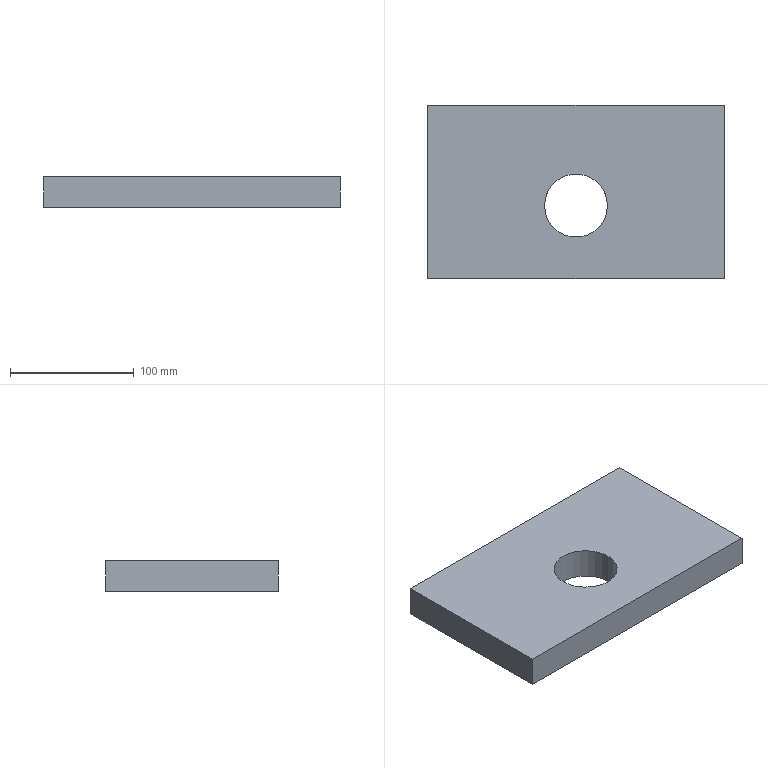Part | SolidWorks | features Extrusion 1 | 1 solid | 8 faces | box 240 x 140 x 25 mm | volume 788929 mm3 | plane 6 | cylinder 2 | commonest cylinder face diameters 51 x2
STEP:
#1=CARTESIAN_POINT('',(94.5,59.,25.));
#2=VERTEX_POINT('',#1);
#3=CARTESIAN_POINT('',(145.5,59.,25.));
#4=VERTEX_POINT('',#3);
#5=CARTESIAN_POINT('',(120.,59.,25.));
#6=DIRECTION('',(0.,0.,1.));
#7=DIRECTION('',(1.,0.,0.));
#8=AXIS2_PLACEMENT_3D('',#5,#6,#7);
#9=CIRCLE('',#8,25.5);
#10=EDGE_CURVE('',#2,#4,#9,.T.);
#11=ORIENTED_EDGE('',*,*,#10,.T.);
#12=CARTESIAN_POINT('',(145.5,59.,0.));
#13=VERTEX_POINT('',#12);
#14=CARTESIAN_POINT('',(145.5,59.,25.));
#15=DIRECTION('',(0.,0.,-1.));
#16=VECTOR('',#15,1000.);
#17=LINE('',#14,#16);
#18=EDGE_CURVE('',#4,#13,#17,.T.);
#19=ORIENTED_EDGE('',*,*,#18,.T.);
#20=CARTESIAN_POINT('',(94.5,59.,0.));
#21=VERTEX_POINT('',#20);
#22=CARTESIAN_POINT('',(120.,59.,0.));
#23=DIRECTION('',(0.,0.,1.));
#24=DIRECTION('',(1.,0.,0.));
#25=AXIS2_PLACEMENT_3D('',#22,#23,#24);
#26=CIRCLE('',#25,25.5);
#27=EDGE_CURVE('',#21,#13,#26,.T.);
#28=ORIENTED_EDGE('',*,*,#27,.F.);
#29=CARTESIAN_POINT('',(94.5,59.,25.));
#30=DIRECTION('',(0.,0.,-1.));
#31=VECTOR('',#30,1000.);
#32=LINE('',#29,#31);
#33=EDGE_CURVE('',#2,#21,#32,.T.);
#34=ORIENTED_EDGE('',*,*,#33,.F.);
#35=EDGE_LOOP('',(#11,#19,#28,#34));
#36=FACE_OUTER_BOUND('',#35,.T.);
#37=CARTESIAN_POINT('',(120.,59.,25.));
#38=DIRECTION('',(0.,0.,-1.));
#39=DIRECTION('',(-1.,0.,0.));
#40=AXIS2_PLACEMENT_3D('',#37,#38,#39);
#41=CYLINDRICAL_SURFACE('',#40,25.5);
#42=ADVANCED_FACE('',(#36),#41,.F.);
#43=CARTESIAN_POINT('',(0.,140.,25.));
#44=VERTEX_POINT('',#43);
#45=CARTESIAN_POINT('',(0.,0.,25.));
#46=VERTEX_POINT('',#45);
#47=CARTESIAN_POINT('',(0.,0.,25.));
#48=DIRECTION('',(0.,-1.,0.));
#49=VECTOR('',#48,1000.);
#50=LINE('',#47,#49);
#51=EDGE_CURVE('',#44,#46,#50,.T.);
#52=ORIENTED_EDGE('',*,*,#51,.T.);
#53=CARTESIAN_POINT('',(240.,0.,25.));
#54=VERTEX_POINT('',#53);
#55=CARTESIAN_POINT('',(0.,0.,25.));
#56=DIRECTION('',(1.,0.,0.));
#57=VECTOR('',#56,1000.);
#58=LINE('',#55,#57);
#59=EDGE_CURVE('',#46,#54,#58,.T.);
#60=ORIENTED_EDGE('',*,*,#59,.T.);
#61=CARTESIAN_POINT('',(240.,140.,25.));
#62=VERTEX_POINT('',#61);
#63=CARTESIAN_POINT('',(240.,0.,25.));
#64=DIRECTION('',(0.,1.,0.));
#65=VECTOR('',#64,1000.);
#66=LINE('',#63,#65);
#67=EDGE_CURVE('',#54,#62,#66,.T.);
#68=ORIENTED_EDGE('',*,*,#67,.T.);
#69=CARTESIAN_POINT('',(0.,140.,25.));
#70=DIRECTION('',(-1.,0.,0.));
#71=VECTOR('',#70,1000.);
#72=LINE('',#69,#71);
#73=EDGE_CURVE('',#62,#44,#72,.T.);
#74=ORIENTED_EDGE('',*,*,#73,.T.);
#75=EDGE_LOOP('',(#52,#60,#68,#74));
#76=FACE_OUTER_BOUND('',#75,.T.);
#77=ORIENTED_EDGE('',*,*,#10,.F.);
#78=CARTESIAN_POINT('',(120.,59.,25.));
#79=DIRECTION('',(0.,0.,1.));
#80=DIRECTION('',(1.,0.,0.));
#81=AXIS2_PLACEMENT_3D('',#78,#79,#80);
#82=CIRCLE('',#81,25.5);
#83=EDGE_CURVE('',#4,#2,#82,.T.);
#84=ORIENTED_EDGE('',*,*,#83,.F.);
#85=EDGE_LOOP('',(#77,#84));
#86=FACE_BOUND('',#85,.T.);
#87=CARTESIAN_POINT('',(0.,0.,25.));
#88=DIRECTION('',(0.,0.,-1.));
#89=DIRECTION('',(-1.,0.,0.));
#90=AXIS2_PLACEMENT_3D('',#87,#88,#89);
#91=PLANE('',#90);
#92=ADVANCED_FACE('',(#76,#86),#91,.F.);
#93=CARTESIAN_POINT('',(0.,140.,0.));
#94=VERTEX_POINT('',#93);
#95=CARTESIAN_POINT('',(0.,0.,0.));
#96=VERTEX_POINT('',#95);
#97=CARTESIAN_POINT('',(0.,0.,0.));
#98=DIRECTION('',(0.,-1.,0.));
#99=VECTOR('',#98,1000.);
#100=LINE('',#97,#99);
#101=EDGE_CURVE('',#94,#96,#100,.T.);
#102=ORIENTED_EDGE('',*,*,#101,.F.);
#103=CARTESIAN_POINT('',(240.,140.,0.));
#104=VERTEX_POINT('',#103);
#105=CARTESIAN_POINT('',(0.,140.,0.));
#106=DIRECTION('',(-1.,0.,0.));
#107=VECTOR('',#106,1000.);
#108=LINE('',#105,#107);
#109=EDGE_CURVE('',#104,#94,#108,.T.);
#110=ORIENTED_EDGE('',*,*,#109,.F.);
#111=CARTESIAN_POINT('',(240.,0.,0.));
#112=VERTEX_POINT('',#111);
#113=CARTESIAN_POINT('',(240.,0.,0.));
#114=DIRECTION('',(0.,1.,0.));
#115=VECTOR('',#114,1000.);
#116=LINE('',#113,#115);
#117=EDGE_CURVE('',#112,#104,#116,.T.);
#118=ORIENTED_EDGE('',*,*,#117,.F.);
#119=CARTESIAN_POINT('',(0.,0.,0.));
#120=DIRECTION('',(1.,0.,0.));
#121=VECTOR('',#120,1000.);
#122=LINE('',#119,#121);
#123=EDGE_CURVE('',#96,#112,#122,.T.);
#124=ORIENTED_EDGE('',*,*,#123,.F.);
#125=EDGE_LOOP('',(#102,#110,#118,#124));
#126=FACE_OUTER_BOUND('',#125,.T.);
#127=ORIENTED_EDGE('',*,*,#27,.T.);
#128=CARTESIAN_POINT('',(120.,59.,0.));
#129=DIRECTION('',(0.,0.,1.));
#130=DIRECTION('',(1.,0.,0.));
#131=AXIS2_PLACEMENT_3D('',#128,#129,#130);
#132=CIRCLE('',#131,25.5);
#133=EDGE_CURVE('',#13,#21,#132,.T.);
#134=ORIENTED_EDGE('',*,*,#133,.T.);
#135=EDGE_LOOP('',(#127,#134));
#136=FACE_BOUND('',#135,.T.);
#137=CARTESIAN_POINT('',(0.,0.,0.));
#138=DIRECTION('',(0.,0.,-1.));
#139=DIRECTION('',(-1.,0.,0.));
#140=AXIS2_PLACEMENT_3D('',#137,#138,#139);
#141=PLANE('',#140);
#142=ADVANCED_FACE('',(#126,#136),#141,.T.);
#143=ORIENTED_EDGE('',*,*,#101,.T.);
#144=CARTESIAN_POINT('',(0.,0.,25.));
#145=DIRECTION('',(0.,0.,-1.));
#146=VECTOR('',#145,1000.);
#147=LINE('',#144,#146);
#148=EDGE_CURVE('',#46,#96,#147,.T.);
#149=ORIENTED_EDGE('',*,*,#148,.F.);
#150=ORIENTED_EDGE('',*,*,#51,.F.);
#151=CARTESIAN_POINT('',(0.,140.,25.));
#152=DIRECTION('',(0.,0.,-1.));
#153=VECTOR('',#152,1000.);
#154=LINE('',#151,#153);
#155=EDGE_CURVE('',#44,#94,#154,.T.);
#156=ORIENTED_EDGE('',*,*,#155,.T.);
#157=EDGE_LOOP('',(#143,#149,#150,#156));
#158=FACE_OUTER_BOUND('',#157,.T.);
#159=CARTESIAN_POINT('',(0.,0.,25.));
#160=DIRECTION('',(1.,0.,0.));
#161=DIRECTION('',(0.,0.,-1.));
#162=AXIS2_PLACEMENT_3D('',#159,#160,#161);
#163=PLANE('',#162);
#164=ADVANCED_FACE('',(#158),#163,.F.);
#165=ORIENTED_EDGE('',*,*,#123,.T.);
#166=CARTESIAN_POINT('',(240.,0.,25.));
#167=DIRECTION('',(0.,0.,-1.));
#168=VECTOR('',#167,1000.);
#169=LINE('',#166,#168);
#170=EDGE_CURVE('',#54,#112,#169,.T.);
#171=ORIENTED_EDGE('',*,*,#170,.F.);
#172=ORIENTED_EDGE('',*,*,#59,.F.);
#173=ORIENTED_EDGE('',*,*,#148,.T.);
#174=EDGE_LOOP('',(#165,#171,#172,#173));
#175=FACE_OUTER_BOUND('',#174,.T.);
#176=CARTESIAN_POINT('',(0.,0.,25.));
#177=DIRECTION('',(0.,1.,0.));
#178=DIRECTION('',(0.,0.,1.));
#179=AXIS2_PLACEMENT_3D('',#176,#177,#178);
#180=PLANE('',#179);
#181=ADVANCED_FACE('',(#175),#180,.F.);
#182=ORIENTED_EDGE('',*,*,#117,.T.);
#183=CARTESIAN_POINT('',(240.,140.,25.));
#184=DIRECTION('',(0.,0.,-1.));
#185=VECTOR('',#184,1000.);
#186=LINE('',#183,#185);
#187=EDGE_CURVE('',#62,#104,#186,.T.);
#188=ORIENTED_EDGE('',*,*,#187,.F.);
#189=ORIENTED_EDGE('',*,*,#67,.F.);
#190=ORIENTED_EDGE('',*,*,#170,.T.);
#191=EDGE_LOOP('',(#182,#188,#189,#190));
#192=FACE_OUTER_BOUND('',#191,.T.);
#193=CARTESIAN_POINT('',(240.,0.,25.));
#194=DIRECTION('',(-1.,0.,0.));
#195=DIRECTION('',(0.,0.,1.));
#196=AXIS2_PLACEMENT_3D('',#193,#194,#195);
#197=PLANE('',#196);
#198=ADVANCED_FACE('',(#192),#197,.F.);
#199=ORIENTED_EDGE('',*,*,#109,.T.);
#200=ORIENTED_EDGE('',*,*,#155,.F.);
#201=ORIENTED_EDGE('',*,*,#73,.F.);
#202=ORIENTED_EDGE('',*,*,#187,.T.);
#203=EDGE_LOOP('',(#199,#200,#201,#202));
#204=FACE_OUTER_BOUND('',#203,.T.);
#205=CARTESIAN_POINT('',(0.,140.,25.));
#206=DIRECTION('',(0.,-1.,0.));
#207=DIRECTION('',(0.,0.,-1.));
#208=AXIS2_PLACEMENT_3D('',#205,#206,#207);
#209=PLANE('',#208);
#210=ADVANCED_FACE('',(#204),#209,.F.);
#211=ORIENTED_EDGE('',*,*,#18,.F.);
#212=ORIENTED_EDGE('',*,*,#83,.T.);
#213=ORIENTED_EDGE('',*,*,#33,.T.);
#214=ORIENTED_EDGE('',*,*,#133,.F.);
#215=EDGE_LOOP('',(#211,#212,#213,#214));
#216=FACE_OUTER_BOUND('',#215,.T.);
#217=CARTESIAN_POINT('',(120.,59.,25.));
#218=DIRECTION('',(0.,0.,-1.));
#219=DIRECTION('',(-1.,0.,0.));
#220=AXIS2_PLACEMENT_3D('',#217,#218,#219);
#221=CYLINDRICAL_SURFACE('',#220,25.5);
#222=ADVANCED_FACE('',(#216),#221,.F.);
#223=CLOSED_SHELL('',(#42,#92,#142,#164,#181,#198,#210,#222));
#224=MANIFOLD_SOLID_BREP('',#223);
#225=CARTESIAN_POINT('',(0.,0.,0.));
#226=DIRECTION('',(0.,0.,1.));
#227=DIRECTION('',(1.,0.,0.));
#228=AXIS2_PLACEMENT_3D('',#225,#226,#227);
#229=(LENGTH_UNIT()NAMED_UNIT(*)SI_UNIT(.MILLI.,.METRE.));
#230=UNCERTAINTY_MEASURE_WITH_UNIT(LENGTH_MEASURE(0.00001),#229,'','');
#231=(NAMED_UNIT(*)PLANE_ANGLE_UNIT()SI_UNIT($,.RADIAN.));
#232=(NAMED_UNIT(*)SI_UNIT($,.STERADIAN.)SOLID_ANGLE_UNIT());
#233=(GEOMETRIC_REPRESENTATION_CONTEXT(3)GLOBAL_UNCERTAINTY_ASSIGNED_CONTEXT((#230))GLOBAL_UNIT_ASSIGNED_CONTEXT((#229,#231,#232))REPRESENTATION_CONTEXT('',''));
#234=ADVANCED_BREP_SHAPE_REPRESENTATION('',(#224,#228),#233);